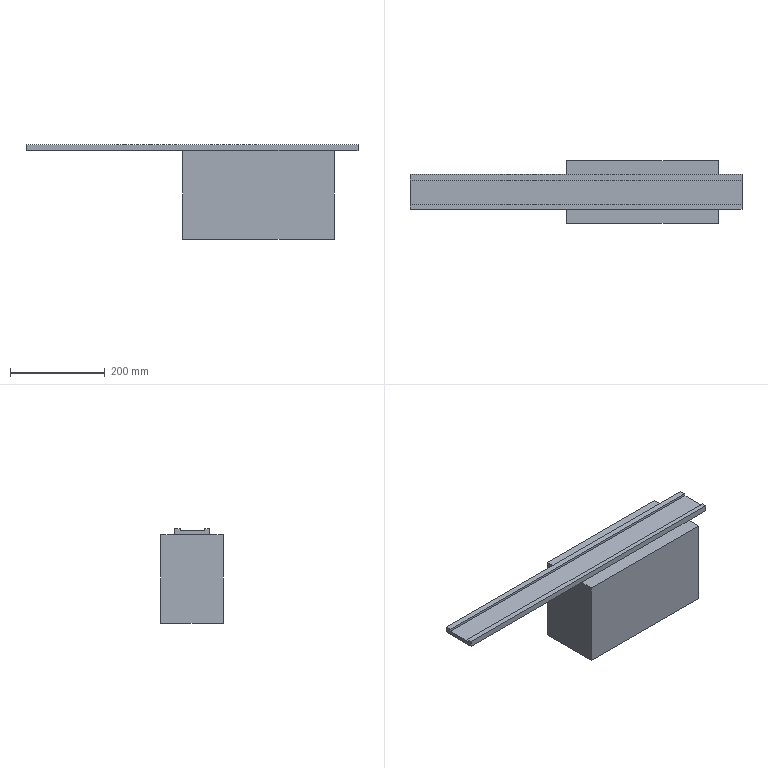Part | STEP file | CALHA_VIBRATORIA_ARRUELA | 1 solid | 26 faces | box 700 x 132 x 200 mm | volume 8382102 mm3 | plane 18 | cone 4 | cylinder 4 | commonest cylinder face diameters 9 x4